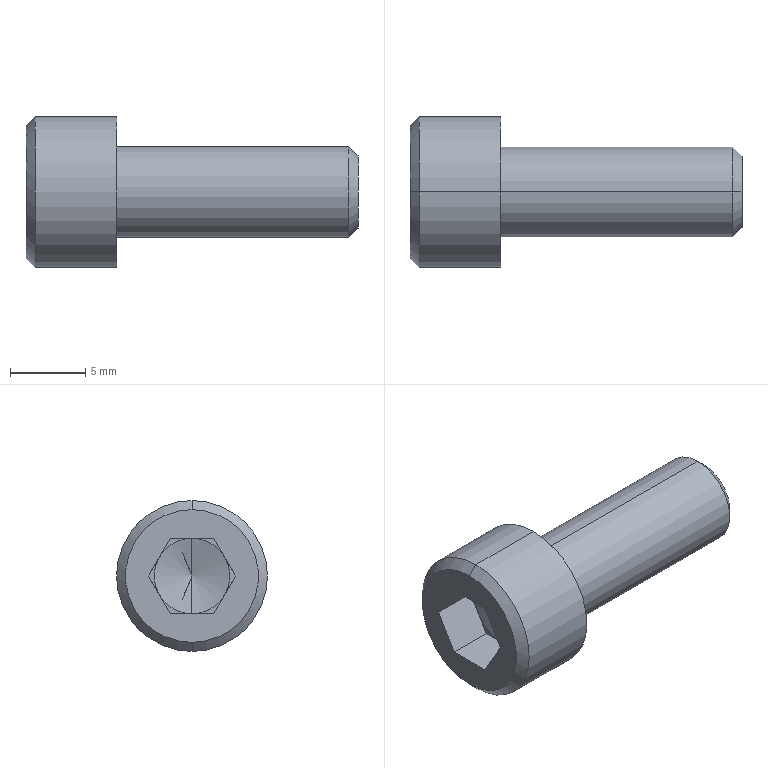Part | STEP file | 0230_310_SCB6-16 | 1 solid | 25 faces | box 22 x 10 x 10 mm | volume 845.558 mm3 | plane 15 | cone 6 | cylinder 4 | commonest cylinder face diameters 6 x2 10 x2